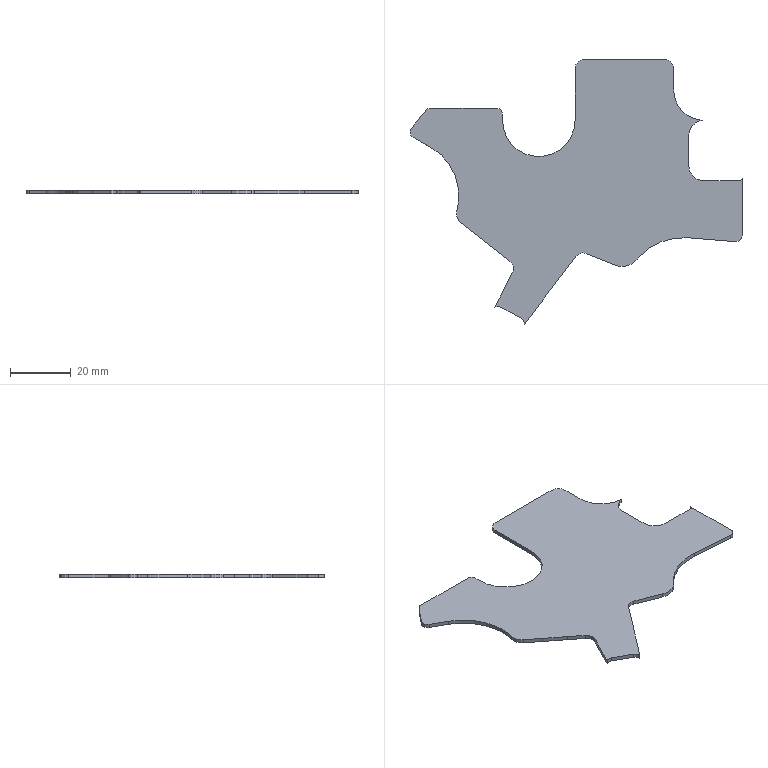Part | STEP file | gslz 2016.10.28-13_id238_x_t | 1 solid | 42 faces | box 109.752 x 87.453 x 1.25 mm | volume 5842 mm3 | plane 21 | cylinder 21 | commonest cylinder face diameters 4 x7 6 x4 10 x2 40 x2 2 x1 8 x1